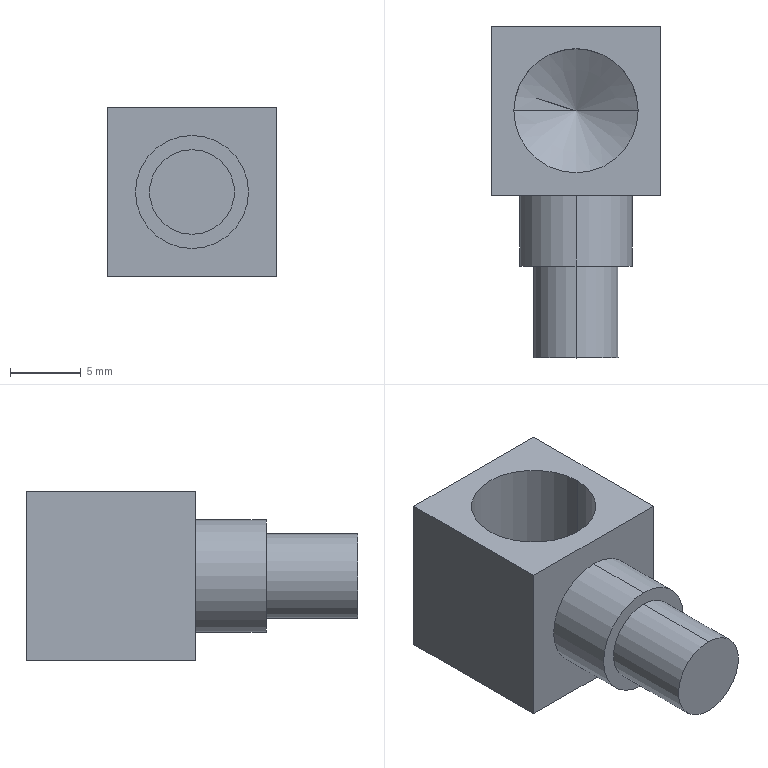Part | STEP file | OL-A | 1 solid | 16 faces | box 12 x 23.5 x 12 mm | volume 1623 mm3 | plane 8 | cylinder 6 | cone 2 | commonest cylinder face diameters 6 x2 8 x2 8.8 x2
STEP:
#1=CARTESIAN_POINT('',(0.,-17.5,3.));
#2=VERTEX_POINT('',#1);
#3=CARTESIAN_POINT('',(0.,-17.5,9.));
#4=VERTEX_POINT('',#3);
#5=CARTESIAN_POINT('',(0.,-17.5,6.));
#6=DIRECTION('',(0.,-1.,0.));
#7=DIRECTION('',(0.,0.,-1.));
#8=AXIS2_PLACEMENT_3D('',#5,#6,#7);
#9=CIRCLE('',#8,3.);
#10=EDGE_CURVE('',#2,#4,#9,.T.);
#11=ORIENTED_EDGE('',*,*,#10,.F.);
#12=CARTESIAN_POINT('',(0.,-11.,3.));
#13=VERTEX_POINT('',#12);
#14=CARTESIAN_POINT('',(0.,-17.5,3.));
#15=DIRECTION('',(0.,1.,0.));
#16=VECTOR('',#15,1000.);
#17=LINE('',#14,#16);
#18=EDGE_CURVE('',#2,#13,#17,.T.);
#19=ORIENTED_EDGE('',*,*,#18,.T.);
#20=CARTESIAN_POINT('',(0.,-11.,9.));
#21=VERTEX_POINT('',#20);
#22=CARTESIAN_POINT('',(0.,-11.,6.));
#23=DIRECTION('',(0.,-1.,0.));
#24=DIRECTION('',(0.,0.,-1.));
#25=AXIS2_PLACEMENT_3D('',#22,#23,#24);
#26=CIRCLE('',#25,3.);
#27=EDGE_CURVE('',#13,#21,#26,.T.);
#28=ORIENTED_EDGE('',*,*,#27,.T.);
#29=CARTESIAN_POINT('',(0.,-17.5,9.));
#30=DIRECTION('',(0.,1.,0.));
#31=VECTOR('',#30,1000.);
#32=LINE('',#29,#31);
#33=EDGE_CURVE('',#4,#21,#32,.T.);
#34=ORIENTED_EDGE('',*,*,#33,.F.);
#35=EDGE_LOOP('',(#11,#19,#28,#34));
#36=FACE_OUTER_BOUND('',#35,.T.);
#37=CARTESIAN_POINT('',(0.,-17.5,6.));
#38=DIRECTION('',(0.,1.,0.));
#39=DIRECTION('',(0.,0.,1.));
#40=AXIS2_PLACEMENT_3D('',#37,#38,#39);
#41=CYLINDRICAL_SURFACE('',#40,3.);
#42=ADVANCED_FACE('',(#36),#41,.T.);
#43=CARTESIAN_POINT('',(0.,-11.,2.));
#44=VERTEX_POINT('',#43);
#45=CARTESIAN_POINT('',(0.,-11.,10.));
#46=VERTEX_POINT('',#45);
#47=CARTESIAN_POINT('',(0.,-11.,6.));
#48=DIRECTION('',(0.,-1.,0.));
#49=DIRECTION('',(0.,0.,-1.));
#50=AXIS2_PLACEMENT_3D('',#47,#48,#49);
#51=CIRCLE('',#50,4.);
#52=EDGE_CURVE('',#44,#46,#51,.T.);
#53=ORIENTED_EDGE('',*,*,#52,.F.);
#54=CARTESIAN_POINT('',(0.,-6.,2.));
#55=VERTEX_POINT('',#54);
#56=CARTESIAN_POINT('',(0.,-11.,2.));
#57=DIRECTION('',(0.,1.,0.));
#58=VECTOR('',#57,1000.);
#59=LINE('',#56,#58);
#60=EDGE_CURVE('',#44,#55,#59,.T.);
#61=ORIENTED_EDGE('',*,*,#60,.T.);
#62=CARTESIAN_POINT('',(0.,-6.,10.));
#63=VERTEX_POINT('',#62);
#64=CARTESIAN_POINT('',(0.,-6.,6.));
#65=DIRECTION('',(0.,-1.,0.));
#66=DIRECTION('',(0.,0.,-1.));
#67=AXIS2_PLACEMENT_3D('',#64,#65,#66);
#68=CIRCLE('',#67,4.);
#69=EDGE_CURVE('',#55,#63,#68,.T.);
#70=ORIENTED_EDGE('',*,*,#69,.T.);
#71=CARTESIAN_POINT('',(0.,-11.,10.));
#72=DIRECTION('',(0.,1.,0.));
#73=VECTOR('',#72,1000.);
#74=LINE('',#71,#73);
#75=EDGE_CURVE('',#46,#63,#74,.T.);
#76=ORIENTED_EDGE('',*,*,#75,.F.);
#77=EDGE_LOOP('',(#53,#61,#70,#76));
#78=FACE_OUTER_BOUND('',#77,.T.);
#79=CARTESIAN_POINT('',(0.,-11.,6.));
#80=DIRECTION('',(0.,1.,0.));
#81=DIRECTION('',(0.,0.,1.));
#82=AXIS2_PLACEMENT_3D('',#79,#80,#81);
#83=CYLINDRICAL_SURFACE('',#82,4.);
#84=ADVANCED_FACE('',(#78),#83,.T.);
#85=CARTESIAN_POINT('',(-4.4,0.,4.));
#86=VERTEX_POINT('',#85);
#87=CARTESIAN_POINT('',(4.4,0.,4.));
#88=VERTEX_POINT('',#87);
#89=CARTESIAN_POINT('',(0.,0.,4.));
#90=DIRECTION('',(0.,0.,1.));
#91=DIRECTION('',(1.,0.,0.));
#92=AXIS2_PLACEMENT_3D('',#89,#90,#91);
#93=CIRCLE('',#92,4.4);
#94=EDGE_CURVE('',#86,#88,#93,.T.);
#95=ORIENTED_EDGE('',*,*,#94,.F.);
#96=CARTESIAN_POINT('',(-4.4,0.,12.));
#97=VERTEX_POINT('',#96);
#98=CARTESIAN_POINT('',(-4.4,0.,12.));
#99=DIRECTION('',(0.,0.,1.));
#100=VECTOR('',#99,1000.);
#101=LINE('',#98,#100);
#102=EDGE_CURVE('',#86,#97,#101,.T.);
#103=ORIENTED_EDGE('',*,*,#102,.T.);
#104=CARTESIAN_POINT('',(4.4,0.,12.));
#105=VERTEX_POINT('',#104);
#106=CARTESIAN_POINT('',(0.,0.,12.));
#107=DIRECTION('',(0.,0.,1.));
#108=DIRECTION('',(1.,0.,0.));
#109=AXIS2_PLACEMENT_3D('',#106,#107,#108);
#110=CIRCLE('',#109,4.4);
#111=EDGE_CURVE('',#97,#105,#110,.T.);
#112=ORIENTED_EDGE('',*,*,#111,.T.);
#113=CARTESIAN_POINT('',(4.4,0.,12.));
#114=DIRECTION('',(0.,0.,1.));
#115=VECTOR('',#114,1000.);
#116=LINE('',#113,#115);
#117=EDGE_CURVE('',#88,#105,#116,.T.);
#118=ORIENTED_EDGE('',*,*,#117,.F.);
#119=EDGE_LOOP('',(#95,#103,#112,#118));
#120=FACE_OUTER_BOUND('',#119,.T.);
#121=CARTESIAN_POINT('',(0.,0.,12.));
#122=DIRECTION('',(0.,0.,1.));
#123=DIRECTION('',(1.,0.,0.));
#124=AXIS2_PLACEMENT_3D('',#121,#122,#123);
#125=CYLINDRICAL_SURFACE('',#124,4.4);
#126=ADVANCED_FACE('',(#120),#125,.F.);
#127=CARTESIAN_POINT('',(0.,0.,1.356));
#128=VERTEX_POINT('',#127);
#129=CARTESIAN_POINT('',(4.4,0.,4.));
#130=DIRECTION('',(0.8572,0.,0.515));
#131=VECTOR('',#130,1000.);
#132=LINE('',#129,#131);
#133=EDGE_CURVE('',#128,#88,#132,.T.);
#134=ORIENTED_EDGE('',*,*,#133,.F.);
#135=CARTESIAN_POINT('',(-4.4,0.,4.));
#136=DIRECTION('',(-0.8572,0.,0.515));
#137=VECTOR('',#136,1000.);
#138=LINE('',#135,#137);
#139=EDGE_CURVE('',#128,#86,#138,.T.);
#140=ORIENTED_EDGE('',*,*,#139,.T.);
#141=ORIENTED_EDGE('',*,*,#94,.T.);
#142=EDGE_LOOP('',(#134,#140,#141));
#143=FACE_OUTER_BOUND('',#142,.T.);
#144=CARTESIAN_POINT('',(0.,0.,4.));
#145=DIRECTION('',(0.,0.,1.));
#146=DIRECTION('',(1.,0.,0.));
#147=AXIS2_PLACEMENT_3D('',#144,#145,#146);
#148=CONICAL_SURFACE('',#147,4.4,1.03);
#149=ADVANCED_FACE('',(#143),#148,.F.);
#150=CARTESIAN_POINT('',(6.,-6.,0.));
#151=VERTEX_POINT('',#150);
#152=CARTESIAN_POINT('',(6.,6.,0.));
#153=VERTEX_POINT('',#152);
#154=CARTESIAN_POINT('',(6.,6.,0.));
#155=DIRECTION('',(0.,1.,0.));
#156=VECTOR('',#155,1000.);
#157=LINE('',#154,#156);
#158=EDGE_CURVE('',#151,#153,#157,.T.);
#159=ORIENTED_EDGE('',*,*,#158,.T.);
#160=CARTESIAN_POINT('',(6.,6.,12.));
#161=VERTEX_POINT('',#160);
#162=CARTESIAN_POINT('',(6.,6.,12.));
#163=DIRECTION('',(0.,0.,-1.));
#164=VECTOR('',#163,1000.);
#165=LINE('',#162,#164);
#166=EDGE_CURVE('',#161,#153,#165,.T.);
#167=ORIENTED_EDGE('',*,*,#166,.F.);
#168=CARTESIAN_POINT('',(6.,-6.,12.));
#169=VERTEX_POINT('',#168);
#170=CARTESIAN_POINT('',(6.,6.,12.));
#171=DIRECTION('',(0.,1.,0.));
#172=VECTOR('',#171,1000.);
#173=LINE('',#170,#172);
#174=EDGE_CURVE('',#169,#161,#173,.T.);
#175=ORIENTED_EDGE('',*,*,#174,.F.);
#176=CARTESIAN_POINT('',(6.,-6.,12.));
#177=DIRECTION('',(0.,0.,-1.));
#178=VECTOR('',#177,1000.);
#179=LINE('',#176,#178);
#180=EDGE_CURVE('',#169,#151,#179,.T.);
#181=ORIENTED_EDGE('',*,*,#180,.T.);
#182=EDGE_LOOP('',(#159,#167,#175,#181));
#183=FACE_OUTER_BOUND('',#182,.T.);
#184=CARTESIAN_POINT('',(6.,6.,12.));
#185=DIRECTION('',(-1.,0.,0.));
#186=DIRECTION('',(0.,-1.,0.));
#187=AXIS2_PLACEMENT_3D('',#184,#185,#186);
#188=PLANE('',#187);
#189=ADVANCED_FACE('',(#183),#188,.F.);
#190=CARTESIAN_POINT('',(-6.,6.,0.));
#191=VERTEX_POINT('',#190);
#192=CARTESIAN_POINT('',(-6.,6.,0.));
#193=DIRECTION('',(-1.,0.,0.));
#194=VECTOR('',#193,1000.);
#195=LINE('',#192,#194);
#196=EDGE_CURVE('',#153,#191,#195,.T.);
#197=ORIENTED_EDGE('',*,*,#196,.T.);
#198=CARTESIAN_POINT('',(-6.,6.,12.));
#199=VERTEX_POINT('',#198);
#200=CARTESIAN_POINT('',(-6.,6.,12.));
#201=DIRECTION('',(0.,0.,-1.));
#202=VECTOR('',#201,1000.);
#203=LINE('',#200,#202);
#204=EDGE_CURVE('',#199,#191,#203,.T.);
#205=ORIENTED_EDGE('',*,*,#204,.F.);
#206=CARTESIAN_POINT('',(-6.,6.,12.));
#207=DIRECTION('',(-1.,0.,0.));
#208=VECTOR('',#207,1000.);
#209=LINE('',#206,#208);
#210=EDGE_CURVE('',#161,#199,#209,.T.);
#211=ORIENTED_EDGE('',*,*,#210,.F.);
#212=ORIENTED_EDGE('',*,*,#166,.T.);
#213=EDGE_LOOP('',(#197,#205,#211,#212));
#214=FACE_OUTER_BOUND('',#213,.T.);
#215=CARTESIAN_POINT('',(-6.,6.,12.));
#216=DIRECTION('',(0.,-1.,0.));
#217=DIRECTION('',(0.,0.,-1.));
#218=AXIS2_PLACEMENT_3D('',#215,#216,#217);
#219=PLANE('',#218);
#220=ADVANCED_FACE('',(#214),#219,.F.);
#221=CARTESIAN_POINT('',(-6.,-6.,0.));
#222=VERTEX_POINT('',#221);
#223=CARTESIAN_POINT('',(-6.,6.,0.));
#224=DIRECTION('',(0.,-1.,0.));
#225=VECTOR('',#224,1000.);
#226=LINE('',#223,#225);
#227=EDGE_CURVE('',#191,#222,#226,.T.);
#228=ORIENTED_EDGE('',*,*,#227,.T.);
#229=CARTESIAN_POINT('',(-6.,-6.,12.));
#230=VERTEX_POINT('',#229);
#231=CARTESIAN_POINT('',(-6.,-6.,12.));
#232=DIRECTION('',(0.,0.,-1.));
#233=VECTOR('',#232,1000.);
#234=LINE('',#231,#233);
#235=EDGE_CURVE('',#230,#222,#234,.T.);
#236=ORIENTED_EDGE('',*,*,#235,.F.);
#237=CARTESIAN_POINT('',(-6.,6.,12.));
#238=DIRECTION('',(0.,-1.,0.));
#239=VECTOR('',#238,1000.);
#240=LINE('',#237,#239);
#241=EDGE_CURVE('',#199,#230,#240,.T.);
#242=ORIENTED_EDGE('',*,*,#241,.F.);
#243=ORIENTED_EDGE('',*,*,#204,.T.);
#244=EDGE_LOOP('',(#228,#236,#242,#243));
#245=FACE_OUTER_BOUND('',#244,.T.);
#246=CARTESIAN_POINT('',(-6.,6.,12.));
#247=DIRECTION('',(1.,0.,0.));
#248=DIRECTION('',(0.,1.,0.));
#249=AXIS2_PLACEMENT_3D('',#246,#247,#248);
#250=PLANE('',#249);
#251=ADVANCED_FACE('',(#245),#250,.F.);
#252=CARTESIAN_POINT('',(0.,-6.,6.));
#253=DIRECTION('',(0.,-1.,0.));
#254=DIRECTION('',(0.,0.,-1.));
#255=AXIS2_PLACEMENT_3D('',#252,#253,#254);
#256=CIRCLE('',#255,4.);
#257=EDGE_CURVE('',#63,#55,#256,.T.);
#258=ORIENTED_EDGE('',*,*,#257,.F.);
#259=ORIENTED_EDGE('',*,*,#69,.F.);
#260=EDGE_LOOP('',(#258,#259));
#261=FACE_BOUND('',#260,.T.);
#262=CARTESIAN_POINT('',(-6.,-6.,0.));
#263=DIRECTION('',(1.,0.,0.));
#264=VECTOR('',#263,1000.);
#265=LINE('',#262,#264);
#266=EDGE_CURVE('',#222,#151,#265,.T.);
#267=ORIENTED_EDGE('',*,*,#266,.T.);
#268=ORIENTED_EDGE('',*,*,#180,.F.);
#269=CARTESIAN_POINT('',(-6.,-6.,12.));
#270=DIRECTION('',(1.,0.,0.));
#271=VECTOR('',#270,1000.);
#272=LINE('',#269,#271);
#273=EDGE_CURVE('',#230,#169,#272,.T.);
#274=ORIENTED_EDGE('',*,*,#273,.F.);
#275=ORIENTED_EDGE('',*,*,#235,.T.);
#276=EDGE_LOOP('',(#267,#268,#274,#275));
#277=FACE_OUTER_BOUND('',#276,.T.);
#278=CARTESIAN_POINT('',(-6.,-6.,12.));
#279=DIRECTION('',(0.,1.,0.));
#280=DIRECTION('',(0.,0.,1.));
#281=AXIS2_PLACEMENT_3D('',#278,#279,#280);
#282=PLANE('',#281);
#283=ADVANCED_FACE('',(#261,#277),#282,.F.);
#284=CARTESIAN_POINT('',(0.,0.,12.));
#285=DIRECTION('',(0.,0.,1.));
#286=DIRECTION('',(1.,0.,0.));
#287=AXIS2_PLACEMENT_3D('',#284,#285,#286);
#288=CIRCLE('',#287,4.4);
#289=EDGE_CURVE('',#105,#97,#288,.T.);
#290=ORIENTED_EDGE('',*,*,#289,.F.);
#291=ORIENTED_EDGE('',*,*,#111,.F.);
#292=EDGE_LOOP('',(#290,#291));
#293=FACE_BOUND('',#292,.T.);
#294=ORIENTED_EDGE('',*,*,#174,.T.);
#295=ORIENTED_EDGE('',*,*,#210,.T.);
#296=ORIENTED_EDGE('',*,*,#241,.T.);
#297=ORIENTED_EDGE('',*,*,#273,.T.);
#298=EDGE_LOOP('',(#294,#295,#296,#297));
#299=FACE_OUTER_BOUND('',#298,.T.);
#300=CARTESIAN_POINT('',(0.,0.,12.));
#301=DIRECTION('',(0.,0.,1.));
#302=DIRECTION('',(1.,0.,0.));
#303=AXIS2_PLACEMENT_3D('',#300,#301,#302);
#304=PLANE('',#303);
#305=ADVANCED_FACE('',(#293,#299),#304,.T.);
#306=ORIENTED_EDGE('',*,*,#158,.F.);
#307=ORIENTED_EDGE('',*,*,#266,.F.);
#308=ORIENTED_EDGE('',*,*,#227,.F.);
#309=ORIENTED_EDGE('',*,*,#196,.F.);
#310=EDGE_LOOP('',(#306,#307,#308,#309));
#311=FACE_OUTER_BOUND('',#310,.T.);
#312=CARTESIAN_POINT('',(0.,0.,0.));
#313=DIRECTION('',(0.,0.,1.));
#314=DIRECTION('',(1.,0.,0.));
#315=AXIS2_PLACEMENT_3D('',#312,#313,#314);
#316=PLANE('',#315);
#317=ADVANCED_FACE('',(#311),#316,.F.);
#318=ORIENTED_EDGE('',*,*,#139,.F.);
#319=ORIENTED_EDGE('',*,*,#133,.T.);
#320=CARTESIAN_POINT('',(0.,0.,4.));
#321=DIRECTION('',(0.,0.,1.));
#322=DIRECTION('',(1.,0.,0.));
#323=AXIS2_PLACEMENT_3D('',#320,#321,#322);
#324=CIRCLE('',#323,4.4);
#325=EDGE_CURVE('',#88,#86,#324,.T.);
#326=ORIENTED_EDGE('',*,*,#325,.T.);
#327=EDGE_LOOP('',(#318,#319,#326));
#328=FACE_OUTER_BOUND('',#327,.T.);
#329=CARTESIAN_POINT('',(0.,0.,4.));
#330=DIRECTION('',(0.,0.,1.));
#331=DIRECTION('',(1.,0.,0.));
#332=AXIS2_PLACEMENT_3D('',#329,#330,#331);
#333=CONICAL_SURFACE('',#332,4.4,1.03);
#334=ADVANCED_FACE('',(#328),#333,.F.);
#335=ORIENTED_EDGE('',*,*,#102,.F.);
#336=ORIENTED_EDGE('',*,*,#325,.F.);
#337=ORIENTED_EDGE('',*,*,#117,.T.);
#338=ORIENTED_EDGE('',*,*,#289,.T.);
#339=EDGE_LOOP('',(#335,#336,#337,#338));
#340=FACE_OUTER_BOUND('',#339,.T.);
#341=CARTESIAN_POINT('',(0.,0.,12.));
#342=DIRECTION('',(0.,0.,1.));
#343=DIRECTION('',(1.,0.,0.));
#344=AXIS2_PLACEMENT_3D('',#341,#342,#343);
#345=CYLINDRICAL_SURFACE('',#344,4.4);
#346=ADVANCED_FACE('',(#340),#345,.F.);
#347=ORIENTED_EDGE('',*,*,#60,.F.);
#348=CARTESIAN_POINT('',(0.,-11.,6.));
#349=DIRECTION('',(0.,-1.,0.));
#350=DIRECTION('',(0.,0.,-1.));
#351=AXIS2_PLACEMENT_3D('',#348,#349,#350);
#352=CIRCLE('',#351,4.);
#353=EDGE_CURVE('',#46,#44,#352,.T.);
#354=ORIENTED_EDGE('',*,*,#353,.F.);
#355=ORIENTED_EDGE('',*,*,#75,.T.);
#356=ORIENTED_EDGE('',*,*,#257,.T.);
#357=EDGE_LOOP('',(#347,#354,#355,#356));
#358=FACE_OUTER_BOUND('',#357,.T.);
#359=CARTESIAN_POINT('',(0.,-11.,6.));
#360=DIRECTION('',(0.,1.,0.));
#361=DIRECTION('',(0.,0.,1.));
#362=AXIS2_PLACEMENT_3D('',#359,#360,#361);
#363=CYLINDRICAL_SURFACE('',#362,4.);
#364=ADVANCED_FACE('',(#358),#363,.T.);
#365=CARTESIAN_POINT('',(0.,-11.,6.));
#366=DIRECTION('',(0.,-1.,0.));
#367=DIRECTION('',(0.,0.,-1.));
#368=AXIS2_PLACEMENT_3D('',#365,#366,#367);
#369=CIRCLE('',#368,3.);
#370=EDGE_CURVE('',#21,#13,#369,.T.);
#371=ORIENTED_EDGE('',*,*,#370,.F.);
#372=ORIENTED_EDGE('',*,*,#27,.F.);
#373=EDGE_LOOP('',(#371,#372));
#374=FACE_BOUND('',#373,.T.);
#375=ORIENTED_EDGE('',*,*,#353,.T.);
#376=ORIENTED_EDGE('',*,*,#52,.T.);
#377=EDGE_LOOP('',(#375,#376));
#378=FACE_OUTER_BOUND('',#377,.T.);
#379=CARTESIAN_POINT('',(0.,-11.,6.));
#380=DIRECTION('',(0.,-1.,0.));
#381=DIRECTION('',(0.,0.,-1.));
#382=AXIS2_PLACEMENT_3D('',#379,#380,#381);
#383=PLANE('',#382);
#384=ADVANCED_FACE('',(#374,#378),#383,.T.);
#385=ORIENTED_EDGE('',*,*,#18,.F.);
#386=CARTESIAN_POINT('',(0.,-17.5,6.));
#387=DIRECTION('',(0.,-1.,0.));
#388=DIRECTION('',(0.,0.,-1.));
#389=AXIS2_PLACEMENT_3D('',#386,#387,#388);
#390=CIRCLE('',#389,3.);
#391=EDGE_CURVE('',#4,#2,#390,.T.);
#392=ORIENTED_EDGE('',*,*,#391,.F.);
#393=ORIENTED_EDGE('',*,*,#33,.T.);
#394=ORIENTED_EDGE('',*,*,#370,.T.);
#395=EDGE_LOOP('',(#385,#392,#393,#394));
#396=FACE_OUTER_BOUND('',#395,.T.);
#397=CARTESIAN_POINT('',(0.,-17.5,6.));
#398=DIRECTION('',(0.,1.,0.));
#399=DIRECTION('',(0.,0.,1.));
#400=AXIS2_PLACEMENT_3D('',#397,#398,#399);
#401=CYLINDRICAL_SURFACE('',#400,3.);
#402=ADVANCED_FACE('',(#396),#401,.T.);
#403=ORIENTED_EDGE('',*,*,#391,.T.);
#404=ORIENTED_EDGE('',*,*,#10,.T.);
#405=EDGE_LOOP('',(#403,#404));
#406=FACE_OUTER_BOUND('',#405,.T.);
#407=CARTESIAN_POINT('',(0.,-17.5,6.));
#408=DIRECTION('',(0.,-1.,0.));
#409=DIRECTION('',(0.,0.,-1.));
#410=AXIS2_PLACEMENT_3D('',#407,#408,#409);
#411=PLANE('',#410);
#412=ADVANCED_FACE('',(#406),#411,.T.);
#413=CLOSED_SHELL('',(#42,#84,#126,#149,#189,#220,#251,#283,#305,#317,#334,#346,#364,#384,#402,#412));
#414=MANIFOLD_SOLID_BREP('',#413);
#415=CARTESIAN_POINT('',(0.,0.,0.));
#416=DIRECTION('',(0.,0.,1.));
#417=DIRECTION('',(1.,0.,0.));
#418=AXIS2_PLACEMENT_3D('',#415,#416,#417);
#419=(LENGTH_UNIT()NAMED_UNIT(*)SI_UNIT(.MILLI.,.METRE.));
#420=UNCERTAINTY_MEASURE_WITH_UNIT(LENGTH_MEASURE(0.00001),#419,'','');
#421=(NAMED_UNIT(*)PLANE_ANGLE_UNIT()SI_UNIT($,.RADIAN.));
#422=(NAMED_UNIT(*)SI_UNIT($,.STERADIAN.)SOLID_ANGLE_UNIT());
#423=(GEOMETRIC_REPRESENTATION_CONTEXT(3)GLOBAL_UNCERTAINTY_ASSIGNED_CONTEXT((#420))GLOBAL_UNIT_ASSIGNED_CONTEXT((#419,#421,#422))REPRESENTATION_CONTEXT('',''));
#424=ADVANCED_BREP_SHAPE_REPRESENTATION('',(#414,#418),#423);